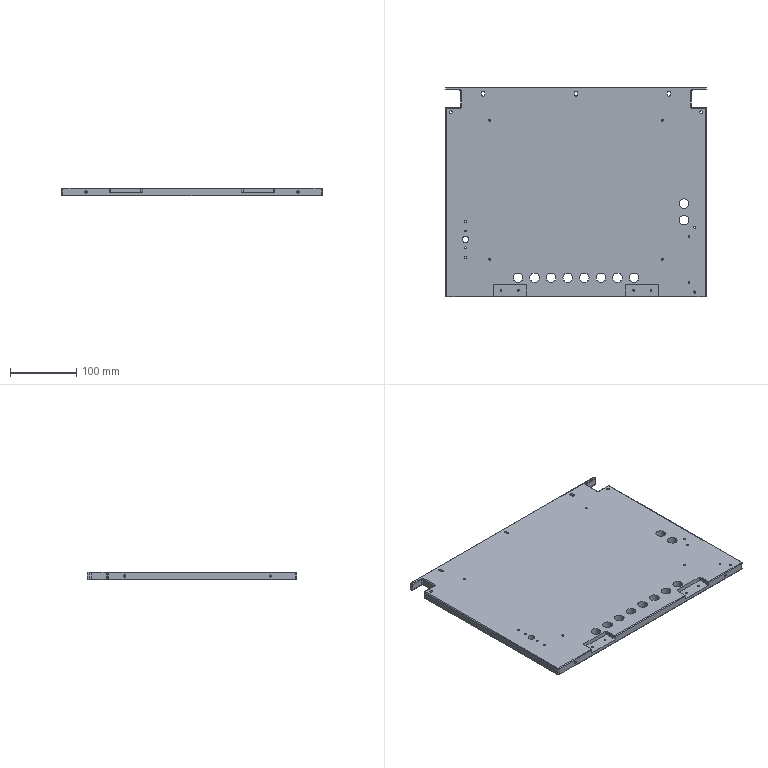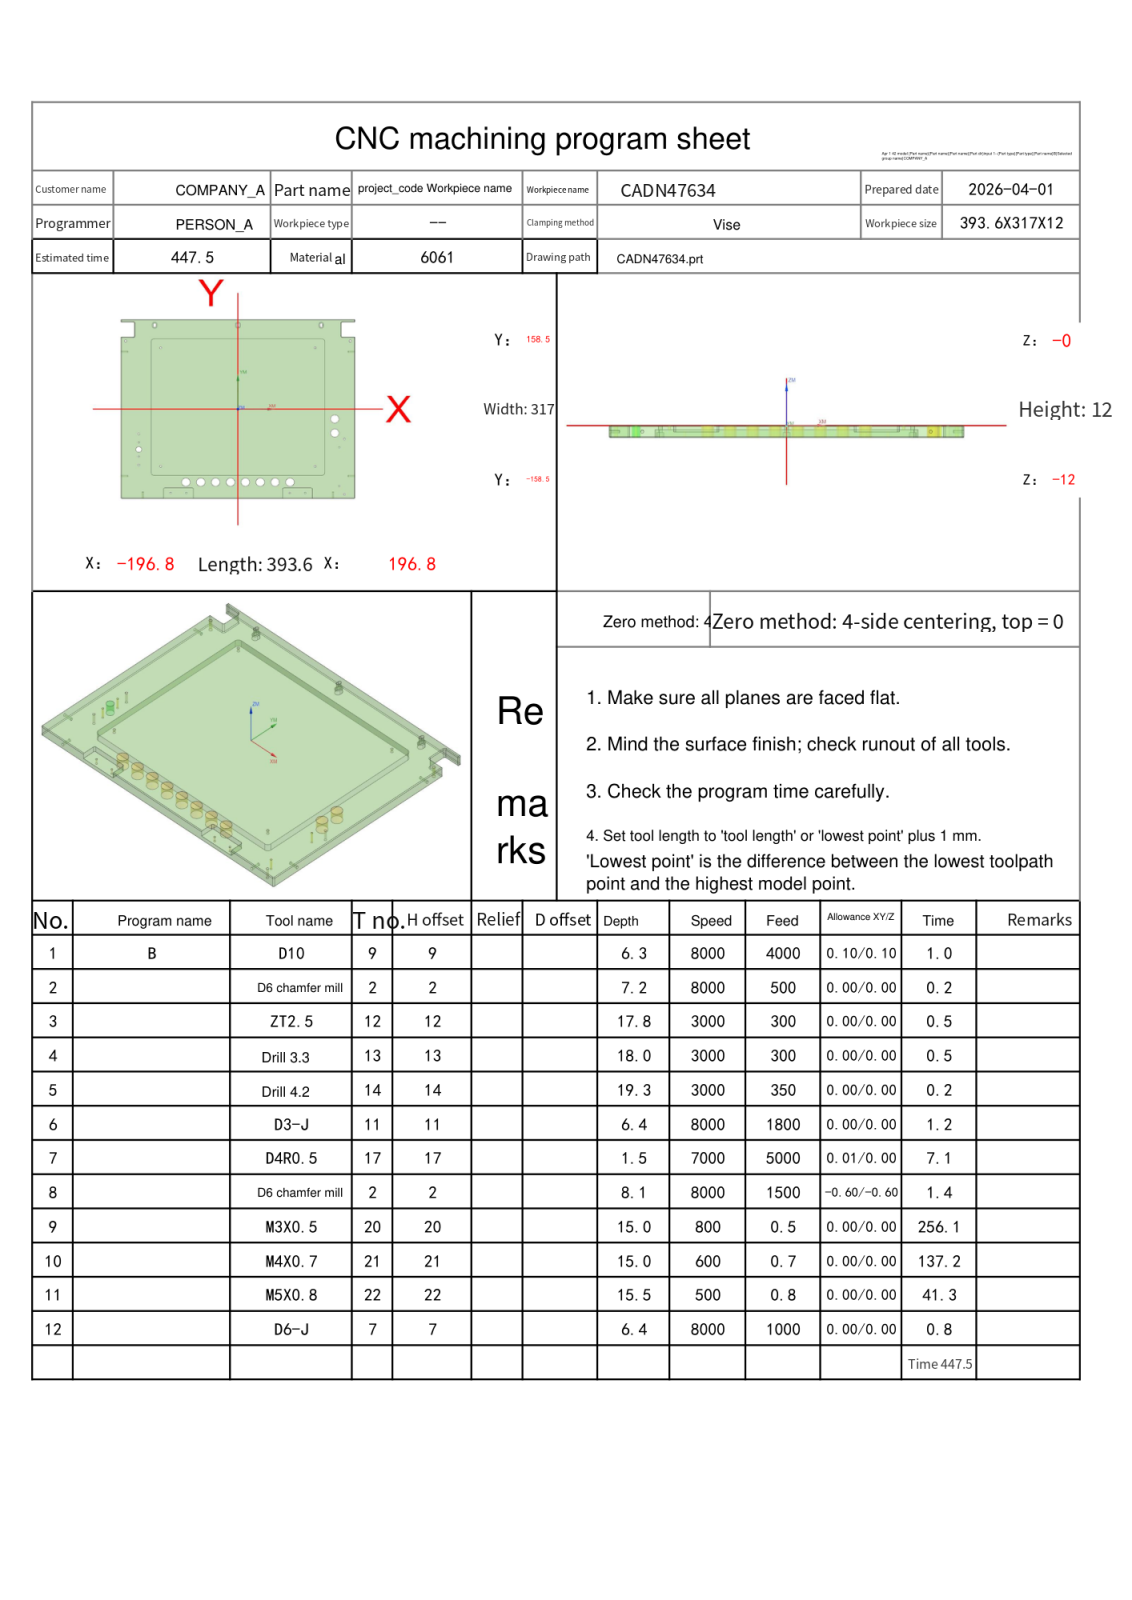NC program | NX | posted by the shop | part box 393.6 x 317 x 12 mm
Lines 1 to 709 of 6733:
%
O0001
(Machine time: 854.18 MIN)
(===Total Tool:11===)
(T9=D10     D=10.  R=0.   D-  H09 Z=-6.3  )
(T2=D6 chamfer mill   D=6.   R=0.   D-  H02 Z=-8.15 )
(T12=ZT2.5  D=2.5  DR_a=118 D-  H12 Z=-17.75)
(T13=Drill 3.3  D=3.3  DR_a=118 D-  H13 Z=-17.99)
(T14=Drill 4.2  D=4.2  DR_a=118 D-  H14 Z=-19.26)
(T11=D3-J   D=3.   R=0.   D-  H11 Z=-6.4  )
(T17=D4R0.5 D=4.   R=0.5  D-  H17 Z=-1.5  )
(T20=M3X0.5 D=2.5  DR_a=180 D-  H20 Z=-15.  )
(T21=M4X0.7 D=3.3  DR_a=180 D-  H21 Z=-15.  )
(T22=M5X0.8 D=4.2  DR_a=180 D-  H22 Z=-15.5 )
(T7=D6-J    D=6.   R=0.   D7  H07 Z=-6.4  )
G80 G90 G17 G49 G40
G91 G28 Z0
M01
N1 T09 M06
(D10  D=10. R=0. H=09 ce=0.10 di=0.10)
G00 G90 G54 X-95.1 Y-166.5 M03 S8000
G43 H09 Z10.1
M08
Z.927
G01 Z-.573 F4000.
Y-163.4
Y-160.598
G03 X-96.098 Y-159.6 I-1. J-.002
G01 X-103.902
G03 X-104.9 Y-160.598 I.002 J-1.
G01 Y-162.4
G02 X-105.9 Y-163.4 I-1. J0.0
G01 X-111.4
G02 X-112.4 Y-162.4 I0.0 J1.
G01 Y-153.098
G02 X-111.402 Y-152.1 I1. J-.002
G01 X-88.598
G02 X-87.6 Y-153.098 I-.002 J-1.
G01 Y-162.544
G03 X-86.754 Y-163.532 I1. J0.0
G01 X-81.254 Y-164.388
X-81.1 Y-164.4
G03 X-80.1 Y-163.4 I0.0 J1.
G01 Y-144.6
X-119.9
Y-163.4
Y-166.504
Z.927
G00 X-95.1 Y-166.5
Z.355
G01 Z-1.145
Y-163.4
Y-160.598
G03 X-96.098 Y-159.6 I-1. J-.002
G01 X-103.902
G03 X-104.9 Y-160.598 I.002 J-1.
G01 Y-162.4
G02 X-105.9 Y-163.4 I-1. J0.0
G01 X-111.4
G02 X-112.4 Y-162.4 I0.0 J1.
G01 Y-153.098
G02 X-111.402 Y-152.1 I1. J-.002
G01 X-88.598
G02 X-87.6 Y-153.098 I-.002 J-1.
G01 Y-162.544
G03 X-86.754 Y-163.532 I1. J0.0
G01 X-81.254 Y-164.388
X-81.1 Y-164.4
G03 X-80.1 Y-163.4 I0.0 J1.
G01 Y-144.6
X-119.9
Y-163.4
Y-166.6
Z.355
G00 X-95.1 Y-166.5
Z-.218
G01 Z-1.718
Y-163.4
Y-160.598
G03 X-96.098 Y-159.6 I-1. J-.002
G01 X-103.902
G03 X-104.9 Y-160.598 I.002 J-1.
G01 Y-162.4
G02 X-105.9 Y-163.4 I-1. J0.0
G01 X-111.4
G02 X-112.4 Y-162.4 I0.0 J1.
G01 Y-153.098
G02 X-111.402 Y-152.1 I1. J-.002
G01 X-88.598
G02 X-87.6 Y-153.098 I-.002 J-1.
G01 Y-162.544
G03 X-86.754 Y-163.532 I1. J0.0
G01 X-81.254 Y-164.388
X-81.1 Y-164.4
G03 X-80.1 Y-163.4 I0.0 J1.
G01 Y-144.6
X-119.9
Y-163.4
Y-166.6
Z-.218
G00 X-95.1 Y-166.5
Z-.791
G01 Z-2.291
Y-163.4
Y-160.598
G03 X-96.098 Y-159.6 I-1. J-.002
G01 X-103.902
G03 X-104.9 Y-160.598 I.002 J-1.
G01 Y-162.4
G02 X-105.9 Y-163.4 I-1. J0.0
G01 X-111.4
G02 X-112.4 Y-162.4 I0.0 J1.
G01 Y-153.098
G02 X-111.402 Y-152.1 I1. J-.002
G01 X-88.598
G02 X-87.6 Y-153.098 I-.002 J-1.
G01 Y-162.544
G03 X-86.754 Y-163.532 I1. J0.0
G01 X-81.254 Y-164.388
X-81.1 Y-164.4
G03 X-80.1 Y-163.4 I0.0 J1.
G01 Y-144.6
X-119.9
Y-163.4
Y-166.6
Z-.791
G00 X-95.1 Y-166.5
Z-1.364
G01 Z-2.864
Y-163.4
Y-160.598
G03 X-96.098 Y-159.6 I-1. J-.002
G01 X-103.902
G03 X-104.9 Y-160.598 I.002 J-1.
G01 Y-162.4
G02 X-105.9 Y-163.4 I-1. J0.0
G01 X-111.4
G02 X-112.4 Y-162.4 I0.0 J1.
G01 Y-153.098
G02 X-111.402 Y-152.1 I1. J-.002
G01 X-88.598
G02 X-87.6 Y-153.098 I-.002 J-1.
G01 Y-162.544
G03 X-86.754 Y-163.532 I1. J0.0
G01 X-81.254 Y-164.388
X-81.1 Y-164.4
G03 X-80.1 Y-163.4 I0.0 J1.
G01 Y-144.6
X-119.9
Y-163.4
Y-166.6
Z-1.364
G00 X-95.1 Y-166.5
Z-1.936
G01 Z-3.436
Y-163.4
Y-160.598
G03 X-96.098 Y-159.6 I-1. J-.002
G01 X-103.902
G03 X-104.9 Y-160.598 I.002 J-1.
G01 Y-162.4
G02 X-105.9 Y-163.4 I-1. J0.0
G01 X-111.4
G02 X-112.4 Y-162.4 I0.0 J1.
G01 Y-153.098
G02 X-111.402 Y-152.1 I1. J-.002
G01 X-88.598
G02 X-87.6 Y-153.098 I-.002 J-1.
G01 Y-162.544
G03 X-86.754 Y-163.532 I1. J0.0
G01 X-81.254 Y-164.388
X-81.1 Y-164.4
G03 X-80.1 Y-163.4 I0.0 J1.
G01 Y-144.6
X-119.9
Y-163.4
Y-166.6
Z-1.936
G00 X-95.1 Y-166.5
Z-2.509
G01 Z-4.009
Y-163.4
Y-160.598
G03 X-96.098 Y-159.6 I-1. J-.002
G01 X-103.902
G03 X-104.9 Y-160.598 I.002 J-1.
G01 Y-162.4
G02 X-105.9 Y-163.4 I-1. J0.0
G01 X-111.4
G02 X-112.4 Y-162.4 I0.0 J1.
G01 Y-153.098
G02 X-111.402 Y-152.1 I1. J-.002
G01 X-88.598
G02 X-87.6 Y-153.098 I-.002 J-1.
G01 Y-162.544
G03 X-86.754 Y-163.532 I1. J0.0
G01 X-81.254 Y-164.388
X-81.1 Y-164.4
G03 X-80.1 Y-163.4 I0.0 J1.
G01 Y-144.6
X-119.9
Y-163.4
Y-166.6
Z-2.509
G00 X-95.1 Y-166.5
Z-3.082
G01 Z-4.582
Y-163.4
Y-160.598
G03 X-96.098 Y-159.6 I-1. J-.002
G01 X-103.902
G03 X-104.9 Y-160.598 I.002 J-1.
G01 Y-162.4
G02 X-105.9 Y-163.4 I-1. J0.0
G01 X-111.4
G02 X-112.4 Y-162.4 I0.0 J1.
G01 Y-153.098
G02 X-111.402 Y-152.1 I1. J-.002
G01 X-88.598
G02 X-87.6 Y-153.098 I-.002 J-1.
G01 Y-162.544
G03 X-86.754 Y-163.532 I1. J0.0
G01 X-81.254 Y-164.388
X-81.1 Y-164.4
G03 X-80.1 Y-163.4 I0.0 J1.
G01 Y-144.6
X-119.9
Y-163.4
Y-166.6
Z-3.082
G00 X-95.1 Y-166.5
Z-3.655
G01 Z-5.155
Y-163.4
Y-160.598
G03 X-96.098 Y-159.6 I-1. J-.002
G01 X-103.902
G03 X-104.9 Y-160.598 I.002 J-1.
G01 Y-162.4
G02 X-105.9 Y-163.4 I-1. J0.0
G01 X-111.4
G02 X-112.4 Y-162.4 I0.0 J1.
G01 Y-153.098
G02 X-111.402 Y-152.1 I1. J-.002
G01 X-88.598
G02 X-87.6 Y-153.098 I-.002 J-1.
G01 Y-162.544
G03 X-86.754 Y-163.532 I1. J0.0
G01 X-81.254 Y-164.388
X-81.1 Y-164.4
G03 X-80.1 Y-163.4 I0.0 J1.
G01 Y-144.6
X-119.9
Y-163.4
Y-166.6
Z-3.655
G00 X-95.1 Y-166.5
Z-4.227
G01 Z-5.727
Y-163.4
Y-160.598
G03 X-96.098 Y-159.6 I-1. J-.002
G01 X-103.902
G03 X-104.9 Y-160.598 I.002 J-1.
G01 Y-162.4
G02 X-105.9 Y-163.4 I-1. J0.0
G01 X-111.4
G02 X-112.4 Y-162.4 I0.0 J1.
G01 Y-153.098
G02 X-111.402 Y-152.1 I1. J-.002
G01 X-88.598
G02 X-87.6 Y-153.098 I-.002 J-1.
G01 Y-162.544
G03 X-86.754 Y-163.532 I1. J0.0
G01 X-81.254 Y-164.388
X-81.1 Y-164.4
G03 X-80.1 Y-163.4 I0.0 J1.
G01 Y-144.6
X-119.9
Y-163.4
Y-166.6
Z-4.227
G00 X-95.1 Y-166.5
Z-4.8
G01 Z-6.3
Y-163.4
Y-160.598
G03 X-96.098 Y-159.6 I-1. J-.002
G01 X-103.902
G03 X-104.9 Y-160.598 I.002 J-1.
G01 Y-162.4
G02 X-105.9 Y-163.4 I-1. J0.0
G01 X-111.4
G02 X-112.4 Y-162.4 I0.0 J1.
G01 Y-153.098
G02 X-111.402 Y-152.1 I1. J-.002
G01 X-88.598
G02 X-87.6 Y-153.098 I-.002 J-1.
G01 Y-162.544
G03 X-86.754 Y-163.532 I1. J0.0
G01 X-81.254 Y-164.388
X-81.1 Y-164.4
G03 X-80.1 Y-163.4 I0.0 J1.
G01 Y-144.6
X-119.9
Y-163.4
Y-166.6
Z-4.8
G00 Z3.
X104.9 Y-166.5
Z.927
G01 Z-.573
Y-163.4
Y-160.598
G03 X103.902 Y-159.6 I-1. J-.002
G01 X96.098
G03 X95.1 Y-160.598 I.002 J-1.
G01 Y-162.4
G02 X94.1 Y-163.4 I-1. J0.0
G01 X88.6
G02 X87.6 Y-162.4 I0.0 J1.
G01 Y-160.598
Y-153.098
G02 X88.598 Y-152.1 I1. J-.002
G01 X111.402
G02 X112.4 Y-153.098 I-.002 J-1.
G01 Y-162.544
G03 X113.246 Y-163.532 I1. J0.0
G01 X118.746 Y-164.388
X118.9 Y-164.4
G03 X119.9 Y-163.4 I0.0 J1.
G01 Y-144.6
X80.1
Y-163.4
Y-166.504
Z.927
G00 X104.9 Y-166.5
Z.355
G01 Z-1.145
Y-163.4
Y-160.598
G03 X103.902 Y-159.6 I-1. J-.002
G01 X96.098
G03 X95.1 Y-160.598 I.002 J-1.
G01 Y-162.4
G02 X94.1 Y-163.4 I-1. J0.0
G01 X88.6
G02 X87.6 Y-162.4 I0.0 J1.
G01 Y-160.598
Y-153.098
G02 X88.598 Y-152.1 I1. J-.002
G01 X111.402
G02 X112.4 Y-153.098 I-.002 J-1.
G01 Y-162.544
G03 X113.246 Y-163.532 I1. J0.0
G01 X118.746 Y-164.388
X118.9 Y-164.4
G03 X119.9 Y-163.4 I0.0 J1.
G01 Y-144.6
X80.1
Y-163.4
Y-166.6
Z.355
G00 X104.9 Y-166.5
Z-.218
G01 Z-1.718
Y-163.4
Y-160.598
G03 X103.902 Y-159.6 I-1. J-.002
G01 X96.098
G03 X95.1 Y-160.598 I.002 J-1.
G01 Y-162.4
G02 X94.1 Y-163.4 I-1. J0.0
G01 X88.6
G02 X87.6 Y-162.4 I0.0 J1.
G01 Y-160.598
Y-153.098
G02 X88.598 Y-152.1 I1. J-.002
G01 X111.402
G02 X112.4 Y-153.098 I-.002 J-1.
G01 Y-162.544
G03 X113.246 Y-163.532 I1. J0.0
G01 X118.746 Y-164.388
X118.9 Y-164.4
G03 X119.9 Y-163.4 I0.0 J1.
G01 Y-144.6
X80.1
Y-163.4
Y-166.6
Z-.218
G00 X104.9 Y-166.5
Z-.791
G01 Z-2.291
Y-163.4
Y-160.598
G03 X103.902 Y-159.6 I-1. J-.002
G01 X96.098
G03 X95.1 Y-160.598 I.002 J-1.
G01 Y-162.4
G02 X94.1 Y-163.4 I-1. J0.0
G01 X88.6
G02 X87.6 Y-162.4 I0.0 J1.
G01 Y-160.598
Y-153.098
G02 X88.598 Y-152.1 I1. J-.002
G01 X111.402
G02 X112.4 Y-153.098 I-.002 J-1.
G01 Y-162.544
G03 X113.246 Y-163.532 I1. J0.0
G01 X118.746 Y-164.388
X118.9 Y-164.4
G03 X119.9 Y-163.4 I0.0 J1.
G01 Y-144.6
X80.1
Y-163.4
Y-166.6
Z-.791
G00 X104.9 Y-166.5
Z-1.364
G01 Z-2.864
Y-163.4
Y-160.598
G03 X103.902 Y-159.6 I-1. J-.002
G01 X96.098
G03 X95.1 Y-160.598 I.002 J-1.
G01 Y-162.4
G02 X94.1 Y-163.4 I-1. J0.0
G01 X88.6
G02 X87.6 Y-162.4 I0.0 J1.
G01 Y-160.598
Y-153.098
G02 X88.598 Y-152.1 I1. J-.002
G01 X111.402
G02 X112.4 Y-153.098 I-.002 J-1.
G01 Y-162.544
G03 X113.246 Y-163.532 I1. J0.0
G01 X118.746 Y-164.388
X118.9 Y-164.4
G03 X119.9 Y-163.4 I0.0 J1.
G01 Y-144.6
X80.1
Y-163.4
Y-166.6
Z-1.364
G00 X104.9 Y-166.5
Z-1.936
G01 Z-3.436
Y-163.4
Y-160.598
G03 X103.902 Y-159.6 I-1. J-.002
G01 X96.098
G03 X95.1 Y-160.598 I.002 J-1.
G01 Y-162.4
G02 X94.1 Y-163.4 I-1. J0.0
G01 X88.6
G02 X87.6 Y-162.4 I0.0 J1.
G01 Y-160.598
Y-153.098
G02 X88.598 Y-152.1 I1. J-.002
G01 X111.402
G02 X112.4 Y-153.098 I-.002 J-1.
G01 Y-162.544
G03 X113.246 Y-163.532 I1. J0.0
G01 X118.746 Y-164.388
X118.9 Y-164.4
G03 X119.9 Y-163.4 I0.0 J1.
G01 Y-144.6
X80.1
Y-163.4
Y-166.6
Z-1.936
G00 X104.9 Y-166.5
Z-2.509
G01 Z-4.009
Y-163.4
Y-160.598
G03 X103.902 Y-159.6 I-1. J-.002
G01 X96.098
G03 X95.1 Y-160.598 I.002 J-1.
G01 Y-162.4
G02 X94.1 Y-163.4 I-1. J0.0
G01 X88.6
G02 X87.6 Y-162.4 I0.0 J1.
G01 Y-160.598
Y-153.098
G02 X88.598 Y-152.1 I1. J-.002
G01 X111.402
G02 X112.4 Y-153.098 I-.002 J-1.
G01 Y-162.544
G03 X113.246 Y-163.532 I1. J0.0
G01 X118.746 Y-164.388
X118.9 Y-164.4
G03 X119.9 Y-163.4 I0.0 J1.
G01 Y-144.6
X80.1
Y-163.4
Y-166.6
Z-2.509
G00 X104.9 Y-166.5
Z-3.082
G01 Z-4.582
Y-163.4
Y-160.598
G03 X103.902 Y-159.6 I-1. J-.002
G01 X96.098
G03 X95.1 Y-160.598 I.002 J-1.
G01 Y-162.4
G02 X94.1 Y-163.4 I-1. J0.0
G01 X88.6
G02 X87.6 Y-162.4 I0.0 J1.
G01 Y-160.598
Y-153.098
G02 X88.598 Y-152.1 I1. J-.002
G01 X111.402
G02 X112.4 Y-153.098 I-.002 J-1.
G01 Y-162.544
G03 X113.246 Y-163.532 I1. J0.0
G01 X118.746 Y-164.388
X118.9 Y-164.4
G03 X119.9 Y-163.4 I0.0 J1.
G01 Y-144.6
X80.1
Y-163.4
Y-166.6
Z-3.082
G00 X104.9 Y-166.5
Z-3.655
G01 Z-5.155
Y-163.4
Y-160.598
G03 X103.902 Y-159.6 I-1. J-.002
G01 X96.098
G03 X95.1 Y-160.598 I.002 J-1.
G01 Y-162.4
G02 X94.1 Y-163.4 I-1. J0.0
G01 X88.6
G02 X87.6 Y-162.4 I0.0 J1.
G01 Y-160.598
Y-153.098
G02 X88.598 Y-152.1 I1. J-.002
G01 X111.402
G02 X112.4 Y-153.098 I-.002 J-1.
G01 Y-162.544
G03 X113.246 Y-163.532 I1. J0.0
G01 X118.746 Y-164.388
X118.9 Y-164.4
G03 X119.9 Y-163.4 I0.0 J1.
G01 Y-144.6
X80.1
Y-163.4
Y-166.6
Z-3.655
G00 X104.9 Y-166.5
Z-4.227
G01 Z-5.727
Y-163.4
Y-160.598
G03 X103.902 Y-159.6 I-1. J-.002
G01 X96.098
G03 X95.1 Y-160.598 I.002 J-1.
G01 Y-162.4
G02 X94.1 Y-163.4 I-1. J0.0
G01 X88.6
G02 X87.6 Y-162.4 I0.0 J1.
G01 Y-160.598
Y-153.098
G02 X88.598 Y-152.1 I1. J-.002
G01 X111.402
G02 X112.4 Y-153.098 I-.002 J-1.
G01 Y-162.544
G03 X113.246 Y-163.532 I1. J0.0
G01 X118.746 Y-164.388
X118.9 Y-164.4
G03 X119.9 Y-163.4 I0.0 J1.
G01 Y-144.6
X80.1
Y-163.4
Y-166.6
Z-4.227
G00 X104.9 Y-166.5
Z-4.8
G01 Z-6.3
Y-163.4
Y-160.598
G03 X103.902 Y-159.6 I-1. J-.002
G01 X96.098
G03 X95.1 Y-160.598 I.002 J-1.
G01 Y-162.4
G02 X94.1 Y-163.4 I-1. J0.0
G01 X88.6
G02 X87.6 Y-162.4 I0.0 J1.
G01 Y-160.598
Y-153.098
G02 X88.598 Y-152.1 I1. J-.002
G01 X111.402
G02 X112.4 Y-153.098 I-.002 J-1.
G01 Y-162.544
G03 X113.246 Y-163.532 I1. J0.0
G01 X118.746 Y-164.388
X118.9 Y-164.4
G03 X119.9 Y-163.4 I0.0 J1.
G01 Y-144.6
X80.1
Y-163.4
Y-166.6
Z-4.8
G00 Z10.1
G91 G28 Z0.0
M05
M09
G91 G28 Z0.0
M01
N2 T02 M06
(D6 chamfer mill D=6. R=0. H=02 ce=0.00 di=0.10)
G00 G90 G54 X188.901 Y120.5 M03 S8000
G43 H02 Z20.
M08
G98 G81 X188.901 Y120.5 Z-.8 R1. F500.
X130. Y108.5
X162.8 Y-17.5
Y-42.5
X179.093 Y-53.06
X170.6 Y-67.62
X130. Y-101.5
X170.6 Y-136.5
X179.093 Y-151.06
X113. Y-148.5 Z-7.2 R-5.4
X87.
X87.5 Y-129.5 Z-.8 R1.
X62.5
X37.5
X12.5
X-12.5
X-37.5
X-62.5
X-87.5
X-87. Y-148.5 Z-7.2 R-5.4
X-113.
X-130. Y-101.5 Z-.8 R1.
X-166.8 Y-99.
Y-84.
Y-71.5
Y-59.
Y-44.
X-130. Y108.5
X-188.901 Y120.5
G80
G00 Z20.
G91 G28 Z0.0
M05
M09
G91 G28 Z0.0
M01
N3 T12 M06
(ZT2.5 D=2.5 DR_a=118 H=12)
G00 G90 G54 X-166.8 Y-59. M03 S3000
G43 H12 Z20.
M08
G98 G83 X-166.8 Y-59. Z-17.751 R1. F300. Q2.
Y-84.
G98 G83 X-113. Y-148.5 Z-17.751 R-5.4 Q2.
X-87.
X87.
X113.
G98 G83 X170.6 Y-136.5 Z-17.751 R1. Q2.
Y-67.62
G80
G00 Z20.
G91 G28 Z0.0
M05
M09
G91 G28 Z0.0
M01
N4 T13 M06
(Drill 3.3 D=3.3 DR_a=118 H=13)
G00 G90 G54 X-130. Y-101.5 M03 S3000
G43 H13 Z20.
M08
G98 G83 X-130. Y-101.5 Z-9.991 R1. F300. Q2.
G98 G83 X-166.8 Y-99. Z-17.991 R1. Q2.
Y-44.
G98 G83 X-130. Y108.5 Z-9.991 R1. Q2.
X130.
G98 G83 X179.093 Y-53.06 Z-17.991 R1. Q2.
G98 G83 X130. Y-101.5 Z-9.991 R1. Q2.
G98 G83 X179.093 Y-151.06 Z-17.991 R1. Q2.
G80
G00 Z20.
G91 G28 Z0.0
M05
M09
G91 G28 Z0.0
M01
N5 T14 M06
(Drill 4.2 D=4.2 DR_a=118 H=14)
G00 G90 G54 X-188.901 Y120.5 M03 S3000
G43 H14 Z20.
M08
G98 G83 X-188.901 Y120.5 Z-19.262 R1. F350. Q3.
X188.901
G80
G00 Z20.
G91 G28 Z0.0
M05
M09
G91 G28 Z0.0
M01